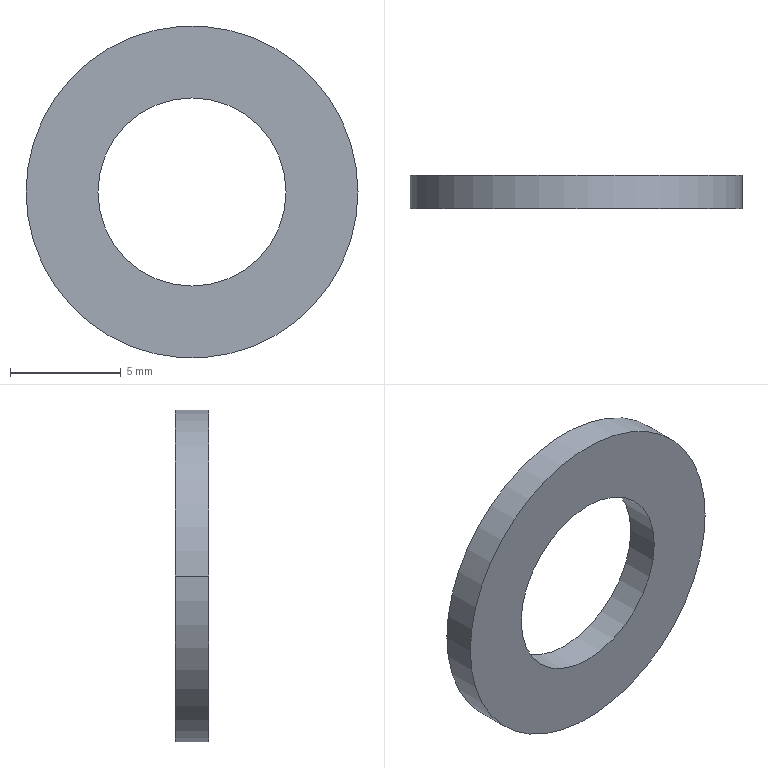Part | STEP file | WSX-SUS-M8X15-1.5 | 1 solid | 6 faces | box 15 x 1.5 x 15 mm | volume 179.954 mm3 | cylinder 4 | plane 2 | commonest cylinder face diameters 8.5 x2 15 x2
STEP:
#1=CARTESIAN_POINT('',(0.,0.,0.));
#2=DIRECTION('',(0.,0.,1.));
#3=DIRECTION('',(1.,0.,0.));
#4=AXIS2_PLACEMENT_3D('',#1,#2,#3);
#5=CARTESIAN_POINT('',(-4.25,0.,0.));
#6=VERTEX_POINT('',#5);
#7=CARTESIAN_POINT('',(-4.25,1.5,0.));
#8=VERTEX_POINT('',#7);
#9=CARTESIAN_POINT('',(-4.25,0.,0.));
#10=DIRECTION('',(0.,1.,0.));
#11=VECTOR('',#10,1.);
#12=LINE('',#9,#11);
#13=CARTESIAN_POINT('',(0.,0.,0.));
#14=DIRECTION('',(0.,1.,0.));
#15=DIRECTION('',(-1.,0.,0.));
#16=AXIS2_PLACEMENT_3D('',#13,#14,#15);
#17=CYLINDRICAL_SURFACE('',#16,4.25);
#18=CARTESIAN_POINT('',(6.283,0.));
#19=DIRECTION('',(0.,1.));
#20=VECTOR('',#19,1.);
#21=LINE('',#18,#20);
#22=(GEOMETRIC_REPRESENTATION_CONTEXT(2)PARAMETRIC_REPRESENTATION_CONTEXT()REPRESENTATION_CONTEXT('',''));
#23=DEFINITIONAL_REPRESENTATION('',(#21),#22);
#24=PCURVE('',#17,#23);
#25=CARTESIAN_POINT('',(0.,0.,0.));
#26=DIRECTION('',(0.,1.,0.));
#27=DIRECTION('',(-1.,0.,0.));
#28=AXIS2_PLACEMENT_3D('',#25,#26,#27);
#29=CYLINDRICAL_SURFACE('',#28,4.25);
#30=CARTESIAN_POINT('',(0.,0.));
#31=DIRECTION('',(0.,1.));
#32=VECTOR('',#31,1.);
#33=LINE('',#30,#32);
#34=(GEOMETRIC_REPRESENTATION_CONTEXT(2)PARAMETRIC_REPRESENTATION_CONTEXT()REPRESENTATION_CONTEXT('',''));
#35=DEFINITIONAL_REPRESENTATION('',(#33),#34);
#36=PCURVE('',#29,#35);
#37=SURFACE_CURVE('',#12,(#24,#36),.PCURVE_S1.);
#38=EDGE_CURVE('',#6,#8,#37,.T.);
#39=ORIENTED_EDGE('',*,*,#38,.T.);
#40=CARTESIAN_POINT('',(4.25,1.5,0.));
#41=VERTEX_POINT('',#40);
#42=CARTESIAN_POINT('',(0.,1.5,0.));
#43=DIRECTION('',(0.,-1.,0.));
#44=DIRECTION('',(1.,0.,0.));
#45=AXIS2_PLACEMENT_3D('',#42,#43,#44);
#46=CIRCLE('',#45,4.25);
#47=CARTESIAN_POINT('',(9.425,1.5));
#48=DIRECTION('',(-1.,0.));
#49=VECTOR('',#48,1.);
#50=LINE('',#47,#49);
#51=(GEOMETRIC_REPRESENTATION_CONTEXT(2)PARAMETRIC_REPRESENTATION_CONTEXT()REPRESENTATION_CONTEXT('',''));
#52=DEFINITIONAL_REPRESENTATION('',(#50),#51);
#53=PCURVE('',#17,#52);
#54=CARTESIAN_POINT('',(0.,1.5,0.));
#55=DIRECTION('',(0.,1.,0.));
#56=DIRECTION('',(-1.,0.,0.));
#57=AXIS2_PLACEMENT_3D('',#54,#55,#56);
#58=PLANE('',#57);
#59=CARTESIAN_POINT('',(-4.25,0.));
#60=CARTESIAN_POINT('',(-4.25,7.361));
#61=CARTESIAN_POINT('',(2.125,3.681));
#62=CARTESIAN_POINT('',(8.5,0.));
#63=CARTESIAN_POINT('',(2.125,-3.681));
#64=CARTESIAN_POINT('',(-4.25,-7.361));
#65=CARTESIAN_POINT('',(-4.25,0.));
#66=(BOUNDED_CURVE()B_SPLINE_CURVE(2,(#59,#60,#61,#62,#63,#64,#65),.UNSPECIFIED.,.T.,.F.)B_SPLINE_CURVE_WITH_KNOTS((1,2,2,2,2,1),(-2.094,0.,2.094,4.189,6.283,8.378),.UNSPECIFIED.)CURVE()GEOMETRIC_REPRESENTATION_ITEM()RATIONAL_B_SPLINE_CURVE((1.,0.5,1.,0.5,1.,0.5,1.))REPRESENTATION_ITEM(''));
#67=(GEOMETRIC_REPRESENTATION_CONTEXT(2)PARAMETRIC_REPRESENTATION_CONTEXT()REPRESENTATION_CONTEXT('',''));
#68=DEFINITIONAL_REPRESENTATION('',(#66),#67);
#69=PCURVE('',#58,#68);
#70=SURFACE_CURVE('',#46,(#53,#69),.PCURVE_S1.);
#71=EDGE_CURVE('',#8,#41,#70,.T.);
#72=ORIENTED_EDGE('',*,*,#71,.T.);
#73=CARTESIAN_POINT('',(4.25,0.,0.));
#74=VERTEX_POINT('',#73);
#75=CARTESIAN_POINT('',(4.25,0.,0.));
#76=DIRECTION('',(0.,1.,0.));
#77=VECTOR('',#76,1.);
#78=LINE('',#75,#77);
#79=CARTESIAN_POINT('',(3.142,0.));
#80=DIRECTION('',(0.,1.));
#81=VECTOR('',#80,1.);
#82=LINE('',#79,#81);
#83=(GEOMETRIC_REPRESENTATION_CONTEXT(2)PARAMETRIC_REPRESENTATION_CONTEXT()REPRESENTATION_CONTEXT('',''));
#84=DEFINITIONAL_REPRESENTATION('',(#82),#83);
#85=PCURVE('',#17,#84);
#86=CARTESIAN_POINT('',(3.142,0.));
#87=DIRECTION('',(0.,1.));
#88=VECTOR('',#87,1.);
#89=LINE('',#86,#88);
#90=(GEOMETRIC_REPRESENTATION_CONTEXT(2)PARAMETRIC_REPRESENTATION_CONTEXT()REPRESENTATION_CONTEXT('',''));
#91=DEFINITIONAL_REPRESENTATION('',(#89),#90);
#92=PCURVE('',#29,#91);
#93=SURFACE_CURVE('',#78,(#85,#92),.PCURVE_S1.);
#94=EDGE_CURVE('',#74,#41,#93,.T.);
#95=ORIENTED_EDGE('',*,*,#94,.F.);
#96=CARTESIAN_POINT('',(0.,0.,0.));
#97=DIRECTION('',(0.,1.,0.));
#98=DIRECTION('',(-1.,0.,0.));
#99=AXIS2_PLACEMENT_3D('',#96,#97,#98);
#100=CIRCLE('',#99,4.25);
#101=CARTESIAN_POINT('',(0.,0.));
#102=DIRECTION('',(1.,0.));
#103=VECTOR('',#102,1.);
#104=LINE('',#101,#103);
#105=(GEOMETRIC_REPRESENTATION_CONTEXT(2)PARAMETRIC_REPRESENTATION_CONTEXT()REPRESENTATION_CONTEXT('',''));
#106=DEFINITIONAL_REPRESENTATION('',(#104),#105);
#107=PCURVE('',#17,#106);
#108=CARTESIAN_POINT('',(0.,0.,0.));
#109=DIRECTION('',(0.,-1.,0.));
#110=DIRECTION('',(1.,0.,0.));
#111=AXIS2_PLACEMENT_3D('',#108,#109,#110);
#112=PLANE('',#111);
#113=CARTESIAN_POINT('',(-4.25,0.));
#114=CARTESIAN_POINT('',(-4.25,7.361));
#115=CARTESIAN_POINT('',(2.125,3.681));
#116=CARTESIAN_POINT('',(8.5,0.));
#117=CARTESIAN_POINT('',(2.125,-3.681));
#118=CARTESIAN_POINT('',(-4.25,-7.361));
#119=CARTESIAN_POINT('',(-4.25,0.));
#120=(BOUNDED_CURVE()B_SPLINE_CURVE(2,(#113,#114,#115,#116,#117,#118,#119),.UNSPECIFIED.,.T.,.F.)B_SPLINE_CURVE_WITH_KNOTS((1,2,2,2,2,1),(-2.094,0.,2.094,4.189,6.283,8.378),.UNSPECIFIED.)CURVE()GEOMETRIC_REPRESENTATION_ITEM()RATIONAL_B_SPLINE_CURVE((1.,0.5,1.,0.5,1.,0.5,1.))REPRESENTATION_ITEM(''));
#121=(GEOMETRIC_REPRESENTATION_CONTEXT(2)PARAMETRIC_REPRESENTATION_CONTEXT()REPRESENTATION_CONTEXT('',''));
#122=DEFINITIONAL_REPRESENTATION('',(#120),#121);
#123=PCURVE('',#112,#122);
#124=SURFACE_CURVE('',#100,(#107,#123),.PCURVE_S1.);
#125=EDGE_CURVE('',#74,#6,#124,.T.);
#126=ORIENTED_EDGE('',*,*,#125,.T.);
#127=EDGE_LOOP('',(#39,#72,#95,#126));
#128=FACE_BOUND('',#127,.F.);
#129=ADVANCED_FACE('',(#128),#17,.F.);
#130=CARTESIAN_POINT('',(-7.5,0.,0.));
#131=VERTEX_POINT('',#130);
#132=CARTESIAN_POINT('',(7.5,0.,0.));
#133=VERTEX_POINT('',#132);
#134=CARTESIAN_POINT('',(0.,0.,0.));
#135=DIRECTION('',(0.,1.,0.));
#136=DIRECTION('',(-1.,0.,0.));
#137=AXIS2_PLACEMENT_3D('',#134,#135,#136);
#138=CIRCLE('',#137,7.5);
#139=CARTESIAN_POINT('',(0.,0.,0.));
#140=DIRECTION('',(0.,1.,0.));
#141=DIRECTION('',(-1.,0.,0.));
#142=AXIS2_PLACEMENT_3D('',#139,#140,#141);
#143=CYLINDRICAL_SURFACE('',#142,7.5);
#144=CARTESIAN_POINT('',(0.,0.));
#145=DIRECTION('',(1.,0.));
#146=VECTOR('',#145,1.);
#147=LINE('',#144,#146);
#148=(GEOMETRIC_REPRESENTATION_CONTEXT(2)PARAMETRIC_REPRESENTATION_CONTEXT()REPRESENTATION_CONTEXT('',''));
#149=DEFINITIONAL_REPRESENTATION('',(#147),#148);
#150=PCURVE('',#143,#149);
#151=CARTESIAN_POINT('',(-7.5,0.));
#152=CARTESIAN_POINT('',(-7.5,12.99));
#153=CARTESIAN_POINT('',(3.75,6.495));
#154=CARTESIAN_POINT('',(15.,0.));
#155=CARTESIAN_POINT('',(3.75,-6.495));
#156=CARTESIAN_POINT('',(-7.5,-12.99));
#157=CARTESIAN_POINT('',(-7.5,0.));
#158=(BOUNDED_CURVE()B_SPLINE_CURVE(2,(#151,#152,#153,#154,#155,#156,#157),.UNSPECIFIED.,.T.,.F.)B_SPLINE_CURVE_WITH_KNOTS((1,2,2,2,2,1),(-2.094,0.,2.094,4.189,6.283,8.378),.UNSPECIFIED.)CURVE()GEOMETRIC_REPRESENTATION_ITEM()RATIONAL_B_SPLINE_CURVE((1.,0.5,1.,0.5,1.,0.5,1.))REPRESENTATION_ITEM(''));
#159=(GEOMETRIC_REPRESENTATION_CONTEXT(2)PARAMETRIC_REPRESENTATION_CONTEXT()REPRESENTATION_CONTEXT('',''));
#160=DEFINITIONAL_REPRESENTATION('',(#158),#159);
#161=PCURVE('',#112,#160);
#162=SURFACE_CURVE('',#138,(#150,#161),.PCURVE_S1.);
#163=EDGE_CURVE('',#131,#133,#162,.T.);
#164=ORIENTED_EDGE('',*,*,#163,.T.);
#165=CARTESIAN_POINT('',(7.5,1.5,0.));
#166=VERTEX_POINT('',#165);
#167=CARTESIAN_POINT('',(7.5,0.,0.));
#168=DIRECTION('',(0.,1.,0.));
#169=VECTOR('',#168,1.);
#170=LINE('',#167,#169);
#171=CARTESIAN_POINT('',(3.142,0.));
#172=DIRECTION('',(0.,1.));
#173=VECTOR('',#172,1.);
#174=LINE('',#171,#173);
#175=(GEOMETRIC_REPRESENTATION_CONTEXT(2)PARAMETRIC_REPRESENTATION_CONTEXT()REPRESENTATION_CONTEXT('',''));
#176=DEFINITIONAL_REPRESENTATION('',(#174),#175);
#177=PCURVE('',#143,#176);
#178=CARTESIAN_POINT('',(0.,0.,0.));
#179=DIRECTION('',(0.,1.,0.));
#180=DIRECTION('',(-1.,0.,0.));
#181=AXIS2_PLACEMENT_3D('',#178,#179,#180);
#182=CYLINDRICAL_SURFACE('',#181,7.5);
#183=CARTESIAN_POINT('',(3.142,0.));
#184=DIRECTION('',(0.,1.));
#185=VECTOR('',#184,1.);
#186=LINE('',#183,#185);
#187=(GEOMETRIC_REPRESENTATION_CONTEXT(2)PARAMETRIC_REPRESENTATION_CONTEXT()REPRESENTATION_CONTEXT('',''));
#188=DEFINITIONAL_REPRESENTATION('',(#186),#187);
#189=PCURVE('',#182,#188);
#190=SURFACE_CURVE('',#170,(#177,#189),.PCURVE_S1.);
#191=EDGE_CURVE('',#133,#166,#190,.T.);
#192=ORIENTED_EDGE('',*,*,#191,.T.);
#193=CARTESIAN_POINT('',(-7.5,1.5,0.));
#194=VERTEX_POINT('',#193);
#195=CARTESIAN_POINT('',(0.,1.5,0.));
#196=DIRECTION('',(0.,-1.,0.));
#197=DIRECTION('',(1.,0.,0.));
#198=AXIS2_PLACEMENT_3D('',#195,#196,#197);
#199=CIRCLE('',#198,7.5);
#200=CARTESIAN_POINT('',(3.142,1.5));
#201=DIRECTION('',(-1.,0.));
#202=VECTOR('',#201,1.);
#203=LINE('',#200,#202);
#204=(GEOMETRIC_REPRESENTATION_CONTEXT(2)PARAMETRIC_REPRESENTATION_CONTEXT()REPRESENTATION_CONTEXT('',''));
#205=DEFINITIONAL_REPRESENTATION('',(#203),#204);
#206=PCURVE('',#143,#205);
#207=CARTESIAN_POINT('',(-7.5,0.));
#208=CARTESIAN_POINT('',(-7.5,12.99));
#209=CARTESIAN_POINT('',(3.75,6.495));
#210=CARTESIAN_POINT('',(15.,0.));
#211=CARTESIAN_POINT('',(3.75,-6.495));
#212=CARTESIAN_POINT('',(-7.5,-12.99));
#213=CARTESIAN_POINT('',(-7.5,0.));
#214=(BOUNDED_CURVE()B_SPLINE_CURVE(2,(#207,#208,#209,#210,#211,#212,#213),.UNSPECIFIED.,.T.,.F.)B_SPLINE_CURVE_WITH_KNOTS((1,2,2,2,2,1),(-2.094,0.,2.094,4.189,6.283,8.378),.UNSPECIFIED.)CURVE()GEOMETRIC_REPRESENTATION_ITEM()RATIONAL_B_SPLINE_CURVE((1.,0.5,1.,0.5,1.,0.5,1.))REPRESENTATION_ITEM(''));
#215=(GEOMETRIC_REPRESENTATION_CONTEXT(2)PARAMETRIC_REPRESENTATION_CONTEXT()REPRESENTATION_CONTEXT('',''));
#216=DEFINITIONAL_REPRESENTATION('',(#214),#215);
#217=PCURVE('',#58,#216);
#218=SURFACE_CURVE('',#199,(#206,#217),.PCURVE_S1.);
#219=EDGE_CURVE('',#166,#194,#218,.T.);
#220=ORIENTED_EDGE('',*,*,#219,.T.);
#221=CARTESIAN_POINT('',(-7.5,0.,0.));
#222=DIRECTION('',(0.,1.,0.));
#223=VECTOR('',#222,1.);
#224=LINE('',#221,#223);
#225=CARTESIAN_POINT('',(0.,0.));
#226=DIRECTION('',(0.,1.));
#227=VECTOR('',#226,1.);
#228=LINE('',#225,#227);
#229=(GEOMETRIC_REPRESENTATION_CONTEXT(2)PARAMETRIC_REPRESENTATION_CONTEXT()REPRESENTATION_CONTEXT('',''));
#230=DEFINITIONAL_REPRESENTATION('',(#228),#229);
#231=PCURVE('',#143,#230);
#232=CARTESIAN_POINT('',(6.283,0.));
#233=DIRECTION('',(0.,1.));
#234=VECTOR('',#233,1.);
#235=LINE('',#232,#234);
#236=(GEOMETRIC_REPRESENTATION_CONTEXT(2)PARAMETRIC_REPRESENTATION_CONTEXT()REPRESENTATION_CONTEXT('',''));
#237=DEFINITIONAL_REPRESENTATION('',(#235),#236);
#238=PCURVE('',#182,#237);
#239=SURFACE_CURVE('',#224,(#231,#238),.PCURVE_S1.);
#240=EDGE_CURVE('',#131,#194,#239,.T.);
#241=ORIENTED_EDGE('',*,*,#240,.F.);
#242=EDGE_LOOP('',(#164,#192,#220,#241));
#243=FACE_BOUND('',#242,.T.);
#244=ADVANCED_FACE('',(#243),#143,.T.);
#245=ORIENTED_EDGE('',*,*,#71,.T.);
#246=CARTESIAN_POINT('',(0.,1.5,0.));
#247=DIRECTION('',(0.,-1.,0.));
#248=DIRECTION('',(1.,0.,0.));
#249=AXIS2_PLACEMENT_3D('',#246,#247,#248);
#250=CIRCLE('',#249,4.25);
#251=CARTESIAN_POINT('',(-4.25,0.));
#252=CARTESIAN_POINT('',(-4.25,7.361));
#253=CARTESIAN_POINT('',(2.125,3.681));
#254=CARTESIAN_POINT('',(8.5,0.));
#255=CARTESIAN_POINT('',(2.125,-3.681));
#256=CARTESIAN_POINT('',(-4.25,-7.361));
#257=CARTESIAN_POINT('',(-4.25,0.));
#258=(BOUNDED_CURVE()B_SPLINE_CURVE(2,(#251,#252,#253,#254,#255,#256,#257),.UNSPECIFIED.,.T.,.F.)B_SPLINE_CURVE_WITH_KNOTS((1,2,2,2,2,1),(-2.094,0.,2.094,4.189,6.283,8.378),.UNSPECIFIED.)CURVE()GEOMETRIC_REPRESENTATION_ITEM()RATIONAL_B_SPLINE_CURVE((1.,0.5,1.,0.5,1.,0.5,1.))REPRESENTATION_ITEM(''));
#259=(GEOMETRIC_REPRESENTATION_CONTEXT(2)PARAMETRIC_REPRESENTATION_CONTEXT()REPRESENTATION_CONTEXT('',''));
#260=DEFINITIONAL_REPRESENTATION('',(#258),#259);
#261=PCURVE('',#58,#260);
#262=CARTESIAN_POINT('',(3.142,1.5));
#263=DIRECTION('',(-1.,0.));
#264=VECTOR('',#263,1.);
#265=LINE('',#262,#264);
#266=(GEOMETRIC_REPRESENTATION_CONTEXT(2)PARAMETRIC_REPRESENTATION_CONTEXT()REPRESENTATION_CONTEXT('',''));
#267=DEFINITIONAL_REPRESENTATION('',(#265),#266);
#268=PCURVE('',#29,#267);
#269=SURFACE_CURVE('',#250,(#261,#268),.PCURVE_S1.);
#270=EDGE_CURVE('',#41,#8,#269,.T.);
#271=ORIENTED_EDGE('',*,*,#270,.T.);
#272=EDGE_LOOP('',(#245,#271));
#273=FACE_BOUND('',#272,.T.);
#274=CARTESIAN_POINT('',(0.,1.5,0.));
#275=DIRECTION('',(0.,-1.,0.));
#276=DIRECTION('',(1.,0.,0.));
#277=AXIS2_PLACEMENT_3D('',#274,#275,#276);
#278=CIRCLE('',#277,7.5);
#279=CARTESIAN_POINT('',(-7.5,0.));
#280=CARTESIAN_POINT('',(-7.5,12.99));
#281=CARTESIAN_POINT('',(3.75,6.495));
#282=CARTESIAN_POINT('',(15.,0.));
#283=CARTESIAN_POINT('',(3.75,-6.495));
#284=CARTESIAN_POINT('',(-7.5,-12.99));
#285=CARTESIAN_POINT('',(-7.5,0.));
#286=(BOUNDED_CURVE()B_SPLINE_CURVE(2,(#279,#280,#281,#282,#283,#284,#285),.UNSPECIFIED.,.T.,.F.)B_SPLINE_CURVE_WITH_KNOTS((1,2,2,2,2,1),(-2.094,0.,2.094,4.189,6.283,8.378),.UNSPECIFIED.)CURVE()GEOMETRIC_REPRESENTATION_ITEM()RATIONAL_B_SPLINE_CURVE((1.,0.5,1.,0.5,1.,0.5,1.))REPRESENTATION_ITEM(''));
#287=(GEOMETRIC_REPRESENTATION_CONTEXT(2)PARAMETRIC_REPRESENTATION_CONTEXT()REPRESENTATION_CONTEXT('',''));
#288=DEFINITIONAL_REPRESENTATION('',(#286),#287);
#289=PCURVE('',#58,#288);
#290=CARTESIAN_POINT('',(9.425,1.5));
#291=DIRECTION('',(-1.,0.));
#292=VECTOR('',#291,1.);
#293=LINE('',#290,#292);
#294=(GEOMETRIC_REPRESENTATION_CONTEXT(2)PARAMETRIC_REPRESENTATION_CONTEXT()REPRESENTATION_CONTEXT('',''));
#295=DEFINITIONAL_REPRESENTATION('',(#293),#294);
#296=PCURVE('',#182,#295);
#297=SURFACE_CURVE('',#278,(#289,#296),.PCURVE_S1.);
#298=EDGE_CURVE('',#194,#166,#297,.T.);
#299=ORIENTED_EDGE('',*,*,#298,.F.);
#300=ORIENTED_EDGE('',*,*,#219,.F.);
#301=EDGE_LOOP('',(#299,#300));
#302=FACE_BOUND('',#301,.T.);
#303=ADVANCED_FACE('',(#273,#302),#58,.T.);
#304=CARTESIAN_POINT('',(0.,0.,0.));
#305=DIRECTION('',(0.,1.,0.));
#306=DIRECTION('',(-1.,0.,0.));
#307=AXIS2_PLACEMENT_3D('',#304,#305,#306);
#308=CIRCLE('',#307,4.25);
#309=CARTESIAN_POINT('',(-4.25,0.));
#310=CARTESIAN_POINT('',(-4.25,7.361));
#311=CARTESIAN_POINT('',(2.125,3.681));
#312=CARTESIAN_POINT('',(8.5,0.));
#313=CARTESIAN_POINT('',(2.125,-3.681));
#314=CARTESIAN_POINT('',(-4.25,-7.361));
#315=CARTESIAN_POINT('',(-4.25,0.));
#316=(BOUNDED_CURVE()B_SPLINE_CURVE(2,(#309,#310,#311,#312,#313,#314,#315),.UNSPECIFIED.,.T.,.F.)B_SPLINE_CURVE_WITH_KNOTS((1,2,2,2,2,1),(-2.094,0.,2.094,4.189,6.283,8.378),.UNSPECIFIED.)CURVE()GEOMETRIC_REPRESENTATION_ITEM()RATIONAL_B_SPLINE_CURVE((1.,0.5,1.,0.5,1.,0.5,1.))REPRESENTATION_ITEM(''));
#317=(GEOMETRIC_REPRESENTATION_CONTEXT(2)PARAMETRIC_REPRESENTATION_CONTEXT()REPRESENTATION_CONTEXT('',''));
#318=DEFINITIONAL_REPRESENTATION('',(#316),#317);
#319=PCURVE('',#112,#318);
#320=CARTESIAN_POINT('',(0.,0.));
#321=DIRECTION('',(1.,0.));
#322=VECTOR('',#321,1.);
#323=LINE('',#320,#322);
#324=(GEOMETRIC_REPRESENTATION_CONTEXT(2)PARAMETRIC_REPRESENTATION_CONTEXT()REPRESENTATION_CONTEXT('',''));
#325=DEFINITIONAL_REPRESENTATION('',(#323),#324);
#326=PCURVE('',#29,#325);
#327=SURFACE_CURVE('',#308,(#319,#326),.PCURVE_S1.);
#328=EDGE_CURVE('',#6,#74,#327,.T.);
#329=ORIENTED_EDGE('',*,*,#328,.T.);
#330=ORIENTED_EDGE('',*,*,#125,.T.);
#331=EDGE_LOOP('',(#329,#330));
#332=FACE_BOUND('',#331,.T.);
#333=ORIENTED_EDGE('',*,*,#163,.F.);
#334=CARTESIAN_POINT('',(0.,0.,0.));
#335=DIRECTION('',(0.,1.,0.));
#336=DIRECTION('',(-1.,0.,0.));
#337=AXIS2_PLACEMENT_3D('',#334,#335,#336);
#338=CIRCLE('',#337,7.5);
#339=CARTESIAN_POINT('',(-7.5,0.));
#340=CARTESIAN_POINT('',(-7.5,12.99));
#341=CARTESIAN_POINT('',(3.75,6.495));
#342=CARTESIAN_POINT('',(15.,0.));
#343=CARTESIAN_POINT('',(3.75,-6.495));
#344=CARTESIAN_POINT('',(-7.5,-12.99));
#345=CARTESIAN_POINT('',(-7.5,0.));
#346=(BOUNDED_CURVE()B_SPLINE_CURVE(2,(#339,#340,#341,#342,#343,#344,#345),.UNSPECIFIED.,.T.,.F.)B_SPLINE_CURVE_WITH_KNOTS((1,2,2,2,2,1),(-2.094,0.,2.094,4.189,6.283,8.378),.UNSPECIFIED.)CURVE()GEOMETRIC_REPRESENTATION_ITEM()RATIONAL_B_SPLINE_CURVE((1.,0.5,1.,0.5,1.,0.5,1.))REPRESENTATION_ITEM(''));
#347=(GEOMETRIC_REPRESENTATION_CONTEXT(2)PARAMETRIC_REPRESENTATION_CONTEXT()REPRESENTATION_CONTEXT('',''));
#348=DEFINITIONAL_REPRESENTATION('',(#346),#347);
#349=PCURVE('',#112,#348);
#350=CARTESIAN_POINT('',(0.,0.));
#351=DIRECTION('',(1.,0.));
#352=VECTOR('',#351,1.);
#353=LINE('',#350,#352);
#354=(GEOMETRIC_REPRESENTATION_CONTEXT(2)PARAMETRIC_REPRESENTATION_CONTEXT()REPRESENTATION_CONTEXT('',''));
#355=DEFINITIONAL_REPRESENTATION('',(#353),#354);
#356=PCURVE('',#182,#355);
#357=SURFACE_CURVE('',#338,(#349,#356),.PCURVE_S1.);
#358=EDGE_CURVE('',#133,#131,#357,.T.);
#359=ORIENTED_EDGE('',*,*,#358,.F.);
#360=EDGE_LOOP('',(#333,#359));
#361=FACE_BOUND('',#360,.T.);
#362=ADVANCED_FACE('',(#332,#361),#112,.T.);
#363=ORIENTED_EDGE('',*,*,#191,.F.);
#364=ORIENTED_EDGE('',*,*,#358,.T.);
#365=ORIENTED_EDGE('',*,*,#240,.T.);
#366=ORIENTED_EDGE('',*,*,#298,.T.);
#367=EDGE_LOOP('',(#363,#364,#365,#366));
#368=FACE_BOUND('',#367,.T.);
#369=ADVANCED_FACE('',(#368),#182,.T.);
#370=ORIENTED_EDGE('',*,*,#270,.T.);
#371=ORIENTED_EDGE('',*,*,#38,.F.);
#372=ORIENTED_EDGE('',*,*,#328,.T.);
#373=ORIENTED_EDGE('',*,*,#94,.T.);
#374=EDGE_LOOP('',(#370,#371,#372,#373));
#375=FACE_BOUND('',#374,.F.);
#376=ADVANCED_FACE('',(#375),#29,.F.);
#377=CLOSED_SHELL('',(#129,#244,#303,#362,#369,#376));
#378=MANIFOLD_SOLID_BREP('',#377);
#379=(LENGTH_UNIT()NAMED_UNIT(*)SI_UNIT(.MILLI.,.METRE.));
#380=UNCERTAINTY_MEASURE_WITH_UNIT(LENGTH_MEASURE(0.0000001),#379,'','');
#381=(NAMED_UNIT(*)PLANE_ANGLE_UNIT()SI_UNIT($,.RADIAN.));
#382=(NAMED_UNIT(*)SI_UNIT($,.STERADIAN.)SOLID_ANGLE_UNIT());
#383=(GEOMETRIC_REPRESENTATION_CONTEXT(3)GLOBAL_UNCERTAINTY_ASSIGNED_CONTEXT((#380))GLOBAL_UNIT_ASSIGNED_CONTEXT((#379,#381,#382))REPRESENTATION_CONTEXT('',''));
#384=ADVANCED_BREP_SHAPE_REPRESENTATION('',(#4,#378),#383);